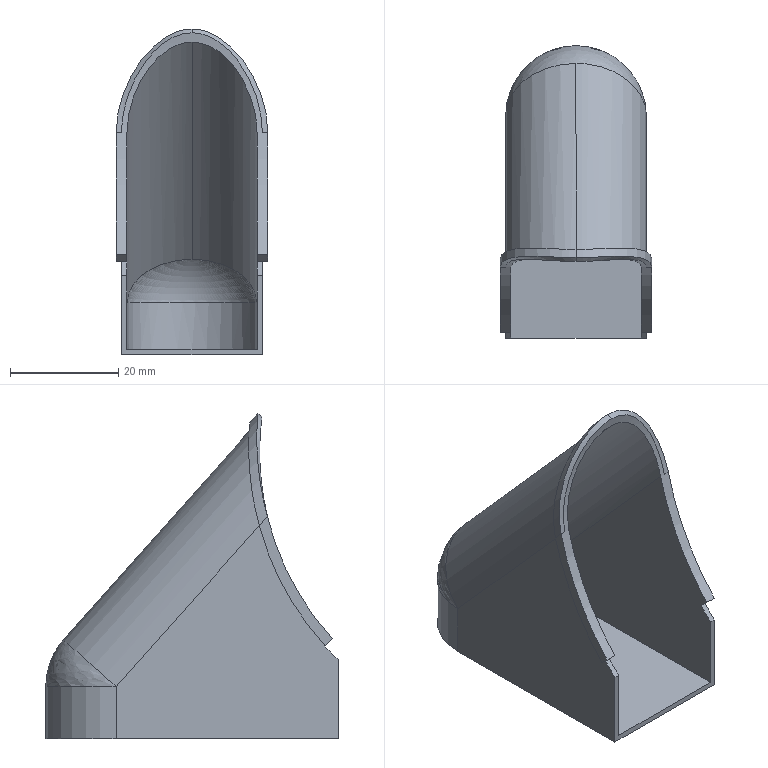Part | STEP file | 1-56.22 | 1 solid | 31 faces | box 28 x 54 x 60.117 mm | volume 6024 mm3 | cylinder 12 | spline 10 | plane 9 | commonest cylinder face diameters 24 x3 26 x3 105.745 x2 106 x2 5 x1 102 x1